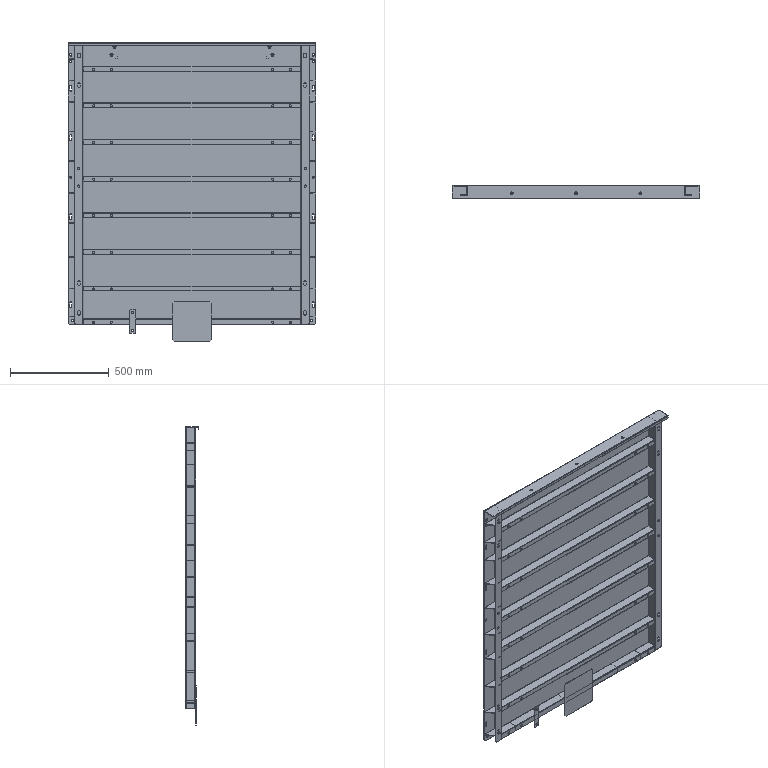Part | SolidWorks | features ReferencePattern 33, LocalLPattern 6, MirrorCompFeat 5 | 48 solids | 1044 faces | box 1250 x 70 x 1510 mm | volume 9091467 mm3 | plane 638 | cylinder 364 | cone 42 | commonest cylinder face diameters 11 x140 10 x82 12 x24 0.4 x22 4.4 x14 6.917 x14